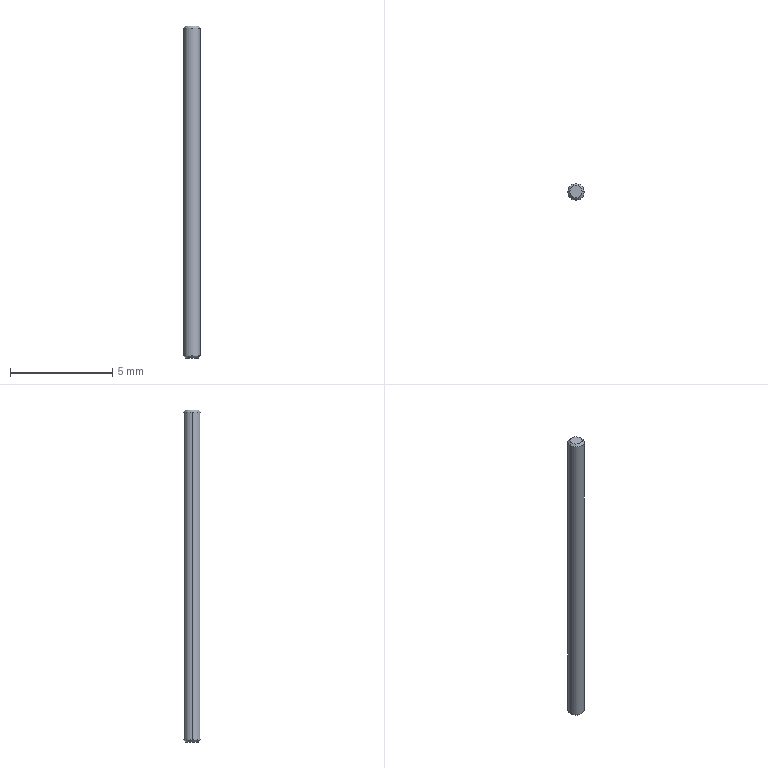Part | SolidWorks | features Chamfer 1, Extrusion 1 | 1 solid | 8 faces | box 0.8 x 0.8 x 16.2 mm | volume 8.12 mm3 | cone 4 | cylinder 2 | plane 2 | commonest cylinder face diameters 0.8 x2
STEP:
#1=CARTESIAN_POINT('',(0.3,0.,16.2));
#2=VERTEX_POINT('',#1);
#3=CARTESIAN_POINT('',(-0.3,0.,16.2));
#4=VERTEX_POINT('',#3);
#5=CARTESIAN_POINT('',(0.,0.,16.2));
#6=DIRECTION('',(0.,0.,1.));
#7=DIRECTION('',(1.,0.,0.));
#8=AXIS2_PLACEMENT_3D('',#5,#6,#7);
#9=CIRCLE('',#8,0.3);
#10=EDGE_CURVE('',#2,#4,#9,.T.);
#11=ORIENTED_EDGE('',*,*,#10,.F.);
#12=CARTESIAN_POINT('',(0.4,0.,16.1));
#13=VERTEX_POINT('',#12);
#14=CARTESIAN_POINT('',(0.3,0.,16.2));
#15=DIRECTION('',(0.7071,0.,-0.7071));
#16=VECTOR('',#15,1000.);
#17=LINE('',#14,#16);
#18=EDGE_CURVE('',#2,#13,#17,.T.);
#19=ORIENTED_EDGE('',*,*,#18,.T.);
#20=CARTESIAN_POINT('',(-0.4,0.,16.1));
#21=VERTEX_POINT('',#20);
#22=CARTESIAN_POINT('',(0.,0.,16.1));
#23=DIRECTION('',(0.,0.,-1.));
#24=DIRECTION('',(1.,0.,0.));
#25=AXIS2_PLACEMENT_3D('',#22,#23,#24);
#26=CIRCLE('',#25,0.4);
#27=EDGE_CURVE('',#21,#13,#26,.T.);
#28=ORIENTED_EDGE('',*,*,#27,.F.);
#29=CARTESIAN_POINT('',(-0.3,0.,16.2));
#30=DIRECTION('',(-0.7071,0.,-0.7071));
#31=VECTOR('',#30,1000.);
#32=LINE('',#29,#31);
#33=EDGE_CURVE('',#4,#21,#32,.T.);
#34=ORIENTED_EDGE('',*,*,#33,.F.);
#35=EDGE_LOOP('',(#11,#19,#28,#34));
#36=FACE_OUTER_BOUND('',#35,.T.);
#37=CARTESIAN_POINT('',(0.,0.,16.2));
#38=DIRECTION('',(0.,0.,-1.));
#39=DIRECTION('',(-1.,0.,0.));
#40=AXIS2_PLACEMENT_3D('',#37,#38,#39);
#41=CONICAL_SURFACE('',#40,0.3,0.7854);
#42=ADVANCED_FACE('',(#36),#41,.T.);
#43=CARTESIAN_POINT('',(-0.3,0.,0.));
#44=VERTEX_POINT('',#43);
#45=CARTESIAN_POINT('',(0.3,0.,0.));
#46=VERTEX_POINT('',#45);
#47=CARTESIAN_POINT('',(0.,0.,0.));
#48=DIRECTION('',(0.,0.,-1.));
#49=DIRECTION('',(1.,0.,0.));
#50=AXIS2_PLACEMENT_3D('',#47,#48,#49);
#51=CIRCLE('',#50,0.3);
#52=EDGE_CURVE('',#44,#46,#51,.T.);
#53=ORIENTED_EDGE('',*,*,#52,.F.);
#54=CARTESIAN_POINT('',(-0.4,0.,0.1));
#55=VERTEX_POINT('',#54);
#56=CARTESIAN_POINT('',(-0.4,0.,0.1));
#57=DIRECTION('',(-0.7071,0.,0.7071));
#58=VECTOR('',#57,1000.);
#59=LINE('',#56,#58);
#60=EDGE_CURVE('',#44,#55,#59,.T.);
#61=ORIENTED_EDGE('',*,*,#60,.T.);
#62=CARTESIAN_POINT('',(0.4,0.,0.1));
#63=VERTEX_POINT('',#62);
#64=CARTESIAN_POINT('',(0.,0.,0.1));
#65=DIRECTION('',(0.,0.,1.));
#66=DIRECTION('',(1.,0.,0.));
#67=AXIS2_PLACEMENT_3D('',#64,#65,#66);
#68=CIRCLE('',#67,0.4);
#69=EDGE_CURVE('',#63,#55,#68,.T.);
#70=ORIENTED_EDGE('',*,*,#69,.F.);
#71=CARTESIAN_POINT('',(0.4,0.,0.1));
#72=DIRECTION('',(0.7071,0.,0.7071));
#73=VECTOR('',#72,1000.);
#74=LINE('',#71,#73);
#75=EDGE_CURVE('',#46,#63,#74,.T.);
#76=ORIENTED_EDGE('',*,*,#75,.F.);
#77=EDGE_LOOP('',(#53,#61,#70,#76));
#78=FACE_OUTER_BOUND('',#77,.T.);
#79=CARTESIAN_POINT('',(0.,0.,0.1));
#80=DIRECTION('',(0.,0.,1.));
#81=DIRECTION('',(1.,0.,0.));
#82=AXIS2_PLACEMENT_3D('',#79,#80,#81);
#83=CONICAL_SURFACE('',#82,0.4,0.7854);
#84=ADVANCED_FACE('',(#78),#83,.T.);
#85=ORIENTED_EDGE('',*,*,#27,.T.);
#86=CARTESIAN_POINT('',(0.4,0.,16.2));
#87=DIRECTION('',(0.,0.,-1.));
#88=VECTOR('',#87,1000.);
#89=LINE('',#86,#88);
#90=EDGE_CURVE('',#13,#63,#89,.T.);
#91=ORIENTED_EDGE('',*,*,#90,.T.);
#92=ORIENTED_EDGE('',*,*,#69,.T.);
#93=CARTESIAN_POINT('',(-0.4,0.,16.2));
#94=DIRECTION('',(0.,0.,-1.));
#95=VECTOR('',#94,1000.);
#96=LINE('',#93,#95);
#97=EDGE_CURVE('',#21,#55,#96,.T.);
#98=ORIENTED_EDGE('',*,*,#97,.F.);
#99=EDGE_LOOP('',(#85,#91,#92,#98));
#100=FACE_OUTER_BOUND('',#99,.T.);
#101=CARTESIAN_POINT('',(0.,0.,16.2));
#102=DIRECTION('',(0.,0.,-1.));
#103=DIRECTION('',(-1.,0.,0.));
#104=AXIS2_PLACEMENT_3D('',#101,#102,#103);
#105=CYLINDRICAL_SURFACE('',#104,0.4);
#106=ADVANCED_FACE('',(#100),#105,.T.);
#107=ORIENTED_EDGE('',*,*,#90,.F.);
#108=CARTESIAN_POINT('',(0.,0.,16.1));
#109=DIRECTION('',(0.,0.,-1.));
#110=DIRECTION('',(1.,0.,0.));
#111=AXIS2_PLACEMENT_3D('',#108,#109,#110);
#112=CIRCLE('',#111,0.4);
#113=EDGE_CURVE('',#13,#21,#112,.T.);
#114=ORIENTED_EDGE('',*,*,#113,.T.);
#115=ORIENTED_EDGE('',*,*,#97,.T.);
#116=CARTESIAN_POINT('',(0.,0.,0.1));
#117=DIRECTION('',(0.,0.,1.));
#118=DIRECTION('',(1.,0.,0.));
#119=AXIS2_PLACEMENT_3D('',#116,#117,#118);
#120=CIRCLE('',#119,0.4);
#121=EDGE_CURVE('',#55,#63,#120,.T.);
#122=ORIENTED_EDGE('',*,*,#121,.T.);
#123=EDGE_LOOP('',(#107,#114,#115,#122));
#124=FACE_OUTER_BOUND('',#123,.T.);
#125=CARTESIAN_POINT('',(0.,0.,16.2));
#126=DIRECTION('',(0.,0.,-1.));
#127=DIRECTION('',(-1.,0.,0.));
#128=AXIS2_PLACEMENT_3D('',#125,#126,#127);
#129=CYLINDRICAL_SURFACE('',#128,0.4);
#130=ADVANCED_FACE('',(#124),#129,.T.);
#131=CARTESIAN_POINT('',(0.,0.,16.2));
#132=DIRECTION('',(0.,0.,1.));
#133=DIRECTION('',(1.,0.,0.));
#134=AXIS2_PLACEMENT_3D('',#131,#132,#133);
#135=CIRCLE('',#134,0.3);
#136=EDGE_CURVE('',#4,#2,#135,.T.);
#137=ORIENTED_EDGE('',*,*,#136,.T.);
#138=ORIENTED_EDGE('',*,*,#10,.T.);
#139=EDGE_LOOP('',(#137,#138));
#140=FACE_OUTER_BOUND('',#139,.T.);
#141=CARTESIAN_POINT('',(0.,0.,16.2));
#142=DIRECTION('',(0.,0.,1.));
#143=DIRECTION('',(1.,0.,0.));
#144=AXIS2_PLACEMENT_3D('',#141,#142,#143);
#145=PLANE('',#144);
#146=ADVANCED_FACE('',(#140),#145,.T.);
#147=CARTESIAN_POINT('',(0.,0.,0.));
#148=DIRECTION('',(0.,0.,-1.));
#149=DIRECTION('',(1.,0.,0.));
#150=AXIS2_PLACEMENT_3D('',#147,#148,#149);
#151=CIRCLE('',#150,0.3);
#152=EDGE_CURVE('',#46,#44,#151,.T.);
#153=ORIENTED_EDGE('',*,*,#152,.T.);
#154=ORIENTED_EDGE('',*,*,#52,.T.);
#155=EDGE_LOOP('',(#153,#154));
#156=FACE_OUTER_BOUND('',#155,.T.);
#157=CARTESIAN_POINT('',(0.,0.,0.));
#158=DIRECTION('',(0.,0.,1.));
#159=DIRECTION('',(1.,0.,0.));
#160=AXIS2_PLACEMENT_3D('',#157,#158,#159);
#161=PLANE('',#160);
#162=ADVANCED_FACE('',(#156),#161,.F.);
#163=ORIENTED_EDGE('',*,*,#60,.F.);
#164=ORIENTED_EDGE('',*,*,#152,.F.);
#165=ORIENTED_EDGE('',*,*,#75,.T.);
#166=ORIENTED_EDGE('',*,*,#121,.F.);
#167=EDGE_LOOP('',(#163,#164,#165,#166));
#168=FACE_OUTER_BOUND('',#167,.T.);
#169=CARTESIAN_POINT('',(0.,0.,0.1));
#170=DIRECTION('',(0.,0.,1.));
#171=DIRECTION('',(1.,0.,0.));
#172=AXIS2_PLACEMENT_3D('',#169,#170,#171);
#173=CONICAL_SURFACE('',#172,0.4,0.7854);
#174=ADVANCED_FACE('',(#168),#173,.T.);
#175=ORIENTED_EDGE('',*,*,#18,.F.);
#176=ORIENTED_EDGE('',*,*,#136,.F.);
#177=ORIENTED_EDGE('',*,*,#33,.T.);
#178=ORIENTED_EDGE('',*,*,#113,.F.);
#179=EDGE_LOOP('',(#175,#176,#177,#178));
#180=FACE_OUTER_BOUND('',#179,.T.);
#181=CARTESIAN_POINT('',(0.,0.,16.2));
#182=DIRECTION('',(0.,0.,-1.));
#183=DIRECTION('',(-1.,0.,0.));
#184=AXIS2_PLACEMENT_3D('',#181,#182,#183);
#185=CONICAL_SURFACE('',#184,0.3,0.7854);
#186=ADVANCED_FACE('',(#180),#185,.T.);
#187=CLOSED_SHELL('',(#42,#84,#106,#130,#146,#162,#174,#186));
#188=MANIFOLD_SOLID_BREP('',#187);
#189=CARTESIAN_POINT('',(0.,0.,0.));
#190=DIRECTION('',(0.,0.,1.));
#191=DIRECTION('',(1.,0.,0.));
#192=AXIS2_PLACEMENT_3D('',#189,#190,#191);
#193=(LENGTH_UNIT()NAMED_UNIT(*)SI_UNIT(.MILLI.,.METRE.));
#194=UNCERTAINTY_MEASURE_WITH_UNIT(LENGTH_MEASURE(0.00001),#193,'','');
#195=(NAMED_UNIT(*)PLANE_ANGLE_UNIT()SI_UNIT($,.RADIAN.));
#196=(NAMED_UNIT(*)SI_UNIT($,.STERADIAN.)SOLID_ANGLE_UNIT());
#197=(GEOMETRIC_REPRESENTATION_CONTEXT(3)GLOBAL_UNCERTAINTY_ASSIGNED_CONTEXT((#194))GLOBAL_UNIT_ASSIGNED_CONTEXT((#193,#195,#196))REPRESENTATION_CONTEXT('',''));
#198=ADVANCED_BREP_SHAPE_REPRESENTATION('',(#188,#192),#197);